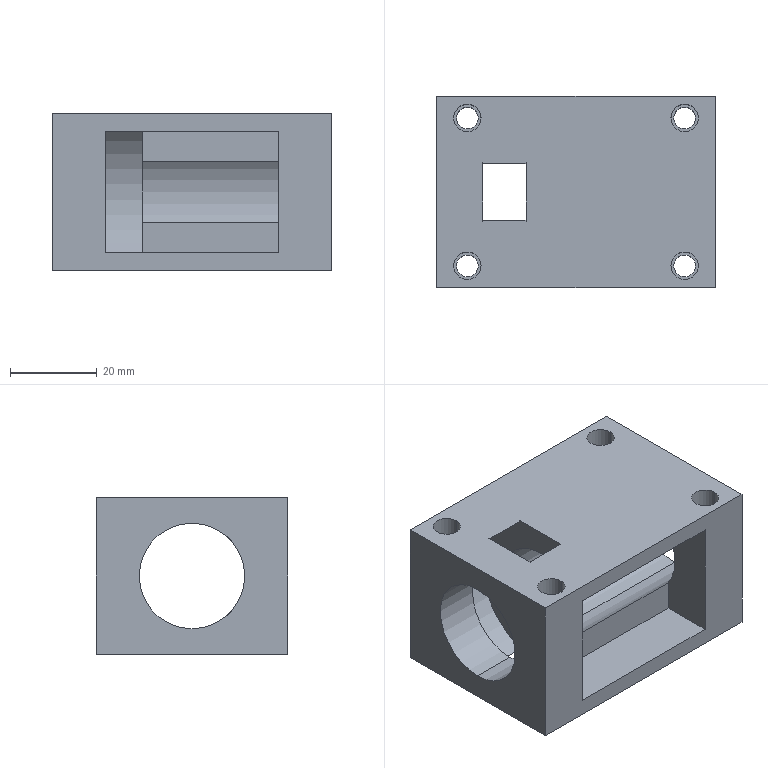Part | SolidWorks | features BaseBody 1 | 1 solid | 40 faces | box 64 x 44 x 36 mm | volume 50225 mm3 | cylinder 22 | plane 18 | commonest cylinder face diameters 5 x8 6.3 x8 24.3 x4 38.3 x2
STEP:
#1=CARTESIAN_POINT('',(-11.5,0.,30.15));
#2=VERTEX_POINT('',#1);
#3=CARTESIAN_POINT('',(-11.5,-10.,24.901));
#4=VERTEX_POINT('',#3);
#5=CARTESIAN_POINT('',(-11.5,0.,18.));
#6=DIRECTION('',(1.,0.,0.));
#7=DIRECTION('',(0.,0.,-1.));
#8=AXIS2_PLACEMENT_3D('',#5,#6,#7);
#9=CIRCLE('',#8,12.15);
#10=EDGE_CURVE('',#2,#4,#9,.T.);
#11=ORIENTED_EDGE('',*,*,#10,.F.);
#12=CARTESIAN_POINT('',(32.,0.,30.15));
#13=VERTEX_POINT('',#12);
#14=CARTESIAN_POINT('',(-33.,0.,30.15));
#15=DIRECTION('',(1.,0.,0.));
#16=VECTOR('',#15,1000.);
#17=LINE('',#14,#16);
#18=EDGE_CURVE('',#2,#13,#17,.T.);
#19=ORIENTED_EDGE('',*,*,#18,.T.);
#20=CARTESIAN_POINT('',(32.,0.,5.85));
#21=VERTEX_POINT('',#20);
#22=CARTESIAN_POINT('',(32.,0.,18.));
#23=DIRECTION('',(-1.,0.,0.));
#24=DIRECTION('',(0.,0.,-1.));
#25=AXIS2_PLACEMENT_3D('',#22,#23,#24);
#26=CIRCLE('',#25,12.15);
#27=EDGE_CURVE('',#21,#13,#26,.T.);
#28=ORIENTED_EDGE('',*,*,#27,.F.);
#29=CARTESIAN_POINT('',(-11.5,0.,5.85));
#30=VERTEX_POINT('',#29);
#31=CARTESIAN_POINT('',(-33.,0.,5.85));
#32=DIRECTION('',(1.,0.,0.));
#33=VECTOR('',#32,1000.);
#34=LINE('',#31,#33);
#35=EDGE_CURVE('',#30,#21,#34,.T.);
#36=ORIENTED_EDGE('',*,*,#35,.F.);
#37=CARTESIAN_POINT('',(-11.5,-10.,11.099));
#38=VERTEX_POINT('',#37);
#39=CARTESIAN_POINT('',(-11.5,0.,18.));
#40=DIRECTION('',(1.,0.,0.));
#41=DIRECTION('',(0.,0.,-1.));
#42=AXIS2_PLACEMENT_3D('',#39,#40,#41);
#43=CIRCLE('',#42,12.15);
#44=EDGE_CURVE('',#38,#30,#43,.T.);
#45=ORIENTED_EDGE('',*,*,#44,.F.);
#46=CARTESIAN_POINT('',(20.,-10.,11.099));
#47=VERTEX_POINT('',#46);
#48=CARTESIAN_POINT('',(-33.,-10.,11.099));
#49=DIRECTION('',(-1.,0.,0.));
#50=VECTOR('',#49,1000.);
#51=LINE('',#48,#50);
#52=EDGE_CURVE('',#47,#38,#51,.T.);
#53=ORIENTED_EDGE('',*,*,#52,.F.);
#54=CARTESIAN_POINT('',(20.,-10.,24.901));
#55=VERTEX_POINT('',#54);
#56=CARTESIAN_POINT('',(20.,0.,18.));
#57=DIRECTION('',(1.,0.,0.));
#58=DIRECTION('',(0.,0.,-1.));
#59=AXIS2_PLACEMENT_3D('',#56,#57,#58);
#60=CIRCLE('',#59,12.15);
#61=EDGE_CURVE('',#55,#47,#60,.T.);
#62=ORIENTED_EDGE('',*,*,#61,.F.);
#63=CARTESIAN_POINT('',(-33.,-10.,24.901));
#64=DIRECTION('',(1.,0.,0.));
#65=VECTOR('',#64,1000.);
#66=LINE('',#63,#65);
#67=EDGE_CURVE('',#4,#55,#66,.T.);
#68=ORIENTED_EDGE('',*,*,#67,.F.);
#69=EDGE_LOOP('',(#11,#19,#28,#36,#45,#53,#62,#68));
#70=FACE_OUTER_BOUND('',#69,.T.);
#71=CARTESIAN_POINT('',(-33.,0.,18.));
#72=DIRECTION('',(1.,0.,0.));
#73=DIRECTION('',(0.,0.,-1.));
#74=AXIS2_PLACEMENT_3D('',#71,#72,#73);
#75=CYLINDRICAL_SURFACE('',#74,12.15);
#76=ADVANCED_FACE('',(#70),#75,.F.);
#77=CARTESIAN_POINT('',(21.85,17.,16.8));
#78=VERTEX_POINT('',#77);
#79=CARTESIAN_POINT('',(28.15,17.,16.8));
#80=VERTEX_POINT('',#79);
#81=CARTESIAN_POINT('',(25.,17.,16.8));
#82=DIRECTION('',(0.,0.,1.));
#83=DIRECTION('',(1.,0.,0.));
#84=AXIS2_PLACEMENT_3D('',#81,#82,#83);
#85=CIRCLE('',#84,3.15);
#86=EDGE_CURVE('',#78,#80,#85,.T.);
#87=ORIENTED_EDGE('',*,*,#86,.F.);
#88=CARTESIAN_POINT('',(21.85,17.,36.));
#89=VERTEX_POINT('',#88);
#90=CARTESIAN_POINT('',(21.85,17.,16.8));
#91=DIRECTION('',(0.,0.,1.));
#92=VECTOR('',#91,1000.);
#93=LINE('',#90,#92);
#94=EDGE_CURVE('',#78,#89,#93,.T.);
#95=ORIENTED_EDGE('',*,*,#94,.T.);
#96=CARTESIAN_POINT('',(28.15,17.,36.));
#97=VERTEX_POINT('',#96);
#98=CARTESIAN_POINT('',(25.,17.,36.));
#99=DIRECTION('',(0.,0.,-1.));
#100=DIRECTION('',(1.,0.,0.));
#101=AXIS2_PLACEMENT_3D('',#98,#99,#100);
#102=CIRCLE('',#101,3.15);
#103=EDGE_CURVE('',#97,#89,#102,.T.);
#104=ORIENTED_EDGE('',*,*,#103,.F.);
#105=CARTESIAN_POINT('',(28.15,17.,16.8));
#106=DIRECTION('',(0.,0.,1.));
#107=VECTOR('',#106,1000.);
#108=LINE('',#105,#107);
#109=EDGE_CURVE('',#80,#97,#108,.T.);
#110=ORIENTED_EDGE('',*,*,#109,.F.);
#111=EDGE_LOOP('',(#87,#95,#104,#110));
#112=FACE_OUTER_BOUND('',#111,.T.);
#113=CARTESIAN_POINT('',(25.,17.,16.8));
#114=DIRECTION('',(0.,0.,1.));
#115=DIRECTION('',(1.,0.,0.));
#116=AXIS2_PLACEMENT_3D('',#113,#114,#115);
#117=CYLINDRICAL_SURFACE('',#116,3.15);
#118=ADVANCED_FACE('',(#112),#117,.F.);
#119=CARTESIAN_POINT('',(-28.15,17.,16.8));
#120=VERTEX_POINT('',#119);
#121=CARTESIAN_POINT('',(-21.85,17.,16.8));
#122=VERTEX_POINT('',#121);
#123=CARTESIAN_POINT('',(-25.,17.,16.8));
#124=DIRECTION('',(0.,0.,1.));
#125=DIRECTION('',(1.,0.,0.));
#126=AXIS2_PLACEMENT_3D('',#123,#124,#125);
#127=CIRCLE('',#126,3.15);
#128=EDGE_CURVE('',#120,#122,#127,.T.);
#129=ORIENTED_EDGE('',*,*,#128,.F.);
#130=CARTESIAN_POINT('',(-28.15,17.,36.));
#131=VERTEX_POINT('',#130);
#132=CARTESIAN_POINT('',(-28.15,17.,16.8));
#133=DIRECTION('',(0.,0.,1.));
#134=VECTOR('',#133,1000.);
#135=LINE('',#132,#134);
#136=EDGE_CURVE('',#120,#131,#135,.T.);
#137=ORIENTED_EDGE('',*,*,#136,.T.);
#138=CARTESIAN_POINT('',(-21.85,17.,36.));
#139=VERTEX_POINT('',#138);
#140=CARTESIAN_POINT('',(-25.,17.,36.));
#141=DIRECTION('',(0.,0.,-1.));
#142=DIRECTION('',(1.,0.,0.));
#143=AXIS2_PLACEMENT_3D('',#140,#141,#142);
#144=CIRCLE('',#143,3.15);
#145=EDGE_CURVE('',#139,#131,#144,.T.);
#146=ORIENTED_EDGE('',*,*,#145,.F.);
#147=CARTESIAN_POINT('',(-21.85,17.,16.8));
#148=DIRECTION('',(0.,0.,1.));
#149=VECTOR('',#148,1000.);
#150=LINE('',#147,#149);
#151=EDGE_CURVE('',#122,#139,#150,.T.);
#152=ORIENTED_EDGE('',*,*,#151,.F.);
#153=EDGE_LOOP('',(#129,#137,#146,#152));
#154=FACE_OUTER_BOUND('',#153,.T.);
#155=CARTESIAN_POINT('',(-25.,17.,16.8));
#156=DIRECTION('',(0.,0.,1.));
#157=DIRECTION('',(1.,0.,0.));
#158=AXIS2_PLACEMENT_3D('',#155,#156,#157);
#159=CYLINDRICAL_SURFACE('',#158,3.15);
#160=ADVANCED_FACE('',(#154),#159,.F.);
#161=CARTESIAN_POINT('',(21.85,-17.,16.8));
#162=VERTEX_POINT('',#161);
#163=CARTESIAN_POINT('',(28.15,-17.,16.8));
#164=VERTEX_POINT('',#163);
#165=CARTESIAN_POINT('',(25.,-17.,16.8));
#166=DIRECTION('',(0.,0.,1.));
#167=DIRECTION('',(1.,0.,0.));
#168=AXIS2_PLACEMENT_3D('',#165,#166,#167);
#169=CIRCLE('',#168,3.15);
#170=EDGE_CURVE('',#162,#164,#169,.T.);
#171=ORIENTED_EDGE('',*,*,#170,.F.);
#172=CARTESIAN_POINT('',(21.85,-17.,36.));
#173=VERTEX_POINT('',#172);
#174=CARTESIAN_POINT('',(21.85,-17.,16.8));
#175=DIRECTION('',(0.,0.,1.));
#176=VECTOR('',#175,1000.);
#177=LINE('',#174,#176);
#178=EDGE_CURVE('',#162,#173,#177,.T.);
#179=ORIENTED_EDGE('',*,*,#178,.T.);
#180=CARTESIAN_POINT('',(28.15,-17.,36.));
#181=VERTEX_POINT('',#180);
#182=CARTESIAN_POINT('',(25.,-17.,36.));
#183=DIRECTION('',(0.,0.,-1.));
#184=DIRECTION('',(1.,0.,0.));
#185=AXIS2_PLACEMENT_3D('',#182,#183,#184);
#186=CIRCLE('',#185,3.15);
#187=EDGE_CURVE('',#181,#173,#186,.T.);
#188=ORIENTED_EDGE('',*,*,#187,.F.);
#189=CARTESIAN_POINT('',(28.15,-17.,16.8));
#190=DIRECTION('',(0.,0.,1.));
#191=VECTOR('',#190,1000.);
#192=LINE('',#189,#191);
#193=EDGE_CURVE('',#164,#181,#192,.T.);
#194=ORIENTED_EDGE('',*,*,#193,.F.);
#195=EDGE_LOOP('',(#171,#179,#188,#194));
#196=FACE_OUTER_BOUND('',#195,.T.);
#197=CARTESIAN_POINT('',(25.,-17.,16.8));
#198=DIRECTION('',(0.,0.,1.));
#199=DIRECTION('',(1.,0.,0.));
#200=AXIS2_PLACEMENT_3D('',#197,#198,#199);
#201=CYLINDRICAL_SURFACE('',#200,3.15);
#202=ADVANCED_FACE('',(#196),#201,.F.);
#203=CARTESIAN_POINT('',(-28.15,-17.,16.8));
#204=VERTEX_POINT('',#203);
#205=CARTESIAN_POINT('',(-21.85,-17.,16.8));
#206=VERTEX_POINT('',#205);
#207=CARTESIAN_POINT('',(-25.,-17.,16.8));
#208=DIRECTION('',(0.,0.,1.));
#209=DIRECTION('',(1.,0.,0.));
#210=AXIS2_PLACEMENT_3D('',#207,#208,#209);
#211=CIRCLE('',#210,3.15);
#212=EDGE_CURVE('',#204,#206,#211,.T.);
#213=ORIENTED_EDGE('',*,*,#212,.F.);
#214=CARTESIAN_POINT('',(-28.15,-17.,36.));
#215=VERTEX_POINT('',#214);
#216=CARTESIAN_POINT('',(-28.15,-17.,16.8));
#217=DIRECTION('',(0.,0.,1.));
#218=VECTOR('',#217,1000.);
#219=LINE('',#216,#218);
#220=EDGE_CURVE('',#204,#215,#219,.T.);
#221=ORIENTED_EDGE('',*,*,#220,.T.);
#222=CARTESIAN_POINT('',(-21.85,-17.,36.));
#223=VERTEX_POINT('',#222);
#224=CARTESIAN_POINT('',(-25.,-17.,36.));
#225=DIRECTION('',(0.,0.,-1.));
#226=DIRECTION('',(1.,0.,0.));
#227=AXIS2_PLACEMENT_3D('',#224,#225,#226);
#228=CIRCLE('',#227,3.15);
#229=EDGE_CURVE('',#223,#215,#228,.T.);
#230=ORIENTED_EDGE('',*,*,#229,.F.);
#231=CARTESIAN_POINT('',(-21.85,-17.,16.8));
#232=DIRECTION('',(0.,0.,1.));
#233=VECTOR('',#232,1000.);
#234=LINE('',#231,#233);
#235=EDGE_CURVE('',#206,#223,#234,.T.);
#236=ORIENTED_EDGE('',*,*,#235,.F.);
#237=EDGE_LOOP('',(#213,#221,#230,#236));
#238=FACE_OUTER_BOUND('',#237,.T.);
#239=CARTESIAN_POINT('',(-25.,-17.,16.8));
#240=DIRECTION('',(0.,0.,1.));
#241=DIRECTION('',(1.,0.,0.));
#242=AXIS2_PLACEMENT_3D('',#239,#240,#241);
#243=CYLINDRICAL_SURFACE('',#242,3.15);
#244=ADVANCED_FACE('',(#238),#243,.F.);
#245=CARTESIAN_POINT('',(27.5,17.,0.));
#246=VERTEX_POINT('',#245);
#247=CARTESIAN_POINT('',(22.5,17.,0.));
#248=VERTEX_POINT('',#247);
#249=CARTESIAN_POINT('',(25.,17.,0.));
#250=DIRECTION('',(0.,0.,-1.));
#251=DIRECTION('',(1.,0.,0.));
#252=AXIS2_PLACEMENT_3D('',#249,#250,#251);
#253=CIRCLE('',#252,2.5);
#254=EDGE_CURVE('',#246,#248,#253,.T.);
#255=ORIENTED_EDGE('',*,*,#254,.T.);
#256=CARTESIAN_POINT('',(22.5,17.,16.8));
#257=VERTEX_POINT('',#256);
#258=CARTESIAN_POINT('',(22.5,17.,-2.));
#259=DIRECTION('',(0.,0.,1.));
#260=VECTOR('',#259,1000.);
#261=LINE('',#258,#260);
#262=EDGE_CURVE('',#248,#257,#261,.T.);
#263=ORIENTED_EDGE('',*,*,#262,.T.);
#264=CARTESIAN_POINT('',(27.5,17.,16.8));
#265=VERTEX_POINT('',#264);
#266=CARTESIAN_POINT('',(25.,17.,16.8));
#267=DIRECTION('',(0.,0.,-1.));
#268=DIRECTION('',(1.,0.,0.));
#269=AXIS2_PLACEMENT_3D('',#266,#267,#268);
#270=CIRCLE('',#269,2.5);
#271=EDGE_CURVE('',#265,#257,#270,.T.);
#272=ORIENTED_EDGE('',*,*,#271,.F.);
#273=CARTESIAN_POINT('',(27.5,17.,-2.));
#274=DIRECTION('',(0.,0.,1.));
#275=VECTOR('',#274,1000.);
#276=LINE('',#273,#275);
#277=EDGE_CURVE('',#246,#265,#276,.T.);
#278=ORIENTED_EDGE('',*,*,#277,.F.);
#279=EDGE_LOOP('',(#255,#263,#272,#278));
#280=FACE_OUTER_BOUND('',#279,.T.);
#281=CARTESIAN_POINT('',(25.,17.,-2.));
#282=DIRECTION('',(0.,0.,1.));
#283=DIRECTION('',(1.,0.,0.));
#284=AXIS2_PLACEMENT_3D('',#281,#282,#283);
#285=CYLINDRICAL_SURFACE('',#284,2.5);
#286=ADVANCED_FACE('',(#280),#285,.F.);
#287=CARTESIAN_POINT('',(-22.5,17.,0.));
#288=VERTEX_POINT('',#287);
#289=CARTESIAN_POINT('',(-27.5,17.,0.));
#290=VERTEX_POINT('',#289);
#291=CARTESIAN_POINT('',(-25.,17.,0.));
#292=DIRECTION('',(0.,0.,-1.));
#293=DIRECTION('',(1.,0.,0.));
#294=AXIS2_PLACEMENT_3D('',#291,#292,#293);
#295=CIRCLE('',#294,2.5);
#296=EDGE_CURVE('',#288,#290,#295,.T.);
#297=ORIENTED_EDGE('',*,*,#296,.T.);
#298=CARTESIAN_POINT('',(-27.5,17.,16.8));
#299=VERTEX_POINT('',#298);
#300=CARTESIAN_POINT('',(-27.5,17.,-2.));
#301=DIRECTION('',(0.,0.,1.));
#302=VECTOR('',#301,1000.);
#303=LINE('',#300,#302);
#304=EDGE_CURVE('',#290,#299,#303,.T.);
#305=ORIENTED_EDGE('',*,*,#304,.T.);
#306=CARTESIAN_POINT('',(-22.5,17.,16.8));
#307=VERTEX_POINT('',#306);
#308=CARTESIAN_POINT('',(-25.,17.,16.8));
#309=DIRECTION('',(0.,0.,-1.));
#310=DIRECTION('',(1.,0.,0.));
#311=AXIS2_PLACEMENT_3D('',#308,#309,#310);
#312=CIRCLE('',#311,2.5);
#313=EDGE_CURVE('',#307,#299,#312,.T.);
#314=ORIENTED_EDGE('',*,*,#313,.F.);
#315=CARTESIAN_POINT('',(-22.5,17.,-2.));
#316=DIRECTION('',(0.,0.,1.));
#317=VECTOR('',#316,1000.);
#318=LINE('',#315,#317);
#319=EDGE_CURVE('',#288,#307,#318,.T.);
#320=ORIENTED_EDGE('',*,*,#319,.F.);
#321=EDGE_LOOP('',(#297,#305,#314,#320));
#322=FACE_OUTER_BOUND('',#321,.T.);
#323=CARTESIAN_POINT('',(-25.,17.,-2.));
#324=DIRECTION('',(0.,0.,1.));
#325=DIRECTION('',(1.,0.,0.));
#326=AXIS2_PLACEMENT_3D('',#323,#324,#325);
#327=CYLINDRICAL_SURFACE('',#326,2.5);
#328=ADVANCED_FACE('',(#322),#327,.F.);
#329=CARTESIAN_POINT('',(27.5,-17.,0.));
#330=VERTEX_POINT('',#329);
#331=CARTESIAN_POINT('',(22.5,-17.,0.));
#332=VERTEX_POINT('',#331);
#333=CARTESIAN_POINT('',(25.,-17.,0.));
#334=DIRECTION('',(0.,0.,-1.));
#335=DIRECTION('',(1.,0.,0.));
#336=AXIS2_PLACEMENT_3D('',#333,#334,#335);
#337=CIRCLE('',#336,2.5);
#338=EDGE_CURVE('',#330,#332,#337,.T.);
#339=ORIENTED_EDGE('',*,*,#338,.T.);
#340=CARTESIAN_POINT('',(22.5,-17.,16.8));
#341=VERTEX_POINT('',#340);
#342=CARTESIAN_POINT('',(22.5,-17.,-2.));
#343=DIRECTION('',(0.,0.,1.));
#344=VECTOR('',#343,1000.);
#345=LINE('',#342,#344);
#346=EDGE_CURVE('',#332,#341,#345,.T.);
#347=ORIENTED_EDGE('',*,*,#346,.T.);
#348=CARTESIAN_POINT('',(27.5,-17.,16.8));
#349=VERTEX_POINT('',#348);
#350=CARTESIAN_POINT('',(25.,-17.,16.8));
#351=DIRECTION('',(0.,0.,-1.));
#352=DIRECTION('',(1.,0.,0.));
#353=AXIS2_PLACEMENT_3D('',#350,#351,#352);
#354=CIRCLE('',#353,2.5);
#355=EDGE_CURVE('',#349,#341,#354,.T.);
#356=ORIENTED_EDGE('',*,*,#355,.F.);
#357=CARTESIAN_POINT('',(27.5,-17.,-2.));
#358=DIRECTION('',(0.,0.,1.));
#359=VECTOR('',#358,1000.);
#360=LINE('',#357,#359);
#361=EDGE_CURVE('',#330,#349,#360,.T.);
#362=ORIENTED_EDGE('',*,*,#361,.F.);
#363=EDGE_LOOP('',(#339,#347,#356,#362));
#364=FACE_OUTER_BOUND('',#363,.T.);
#365=CARTESIAN_POINT('',(25.,-17.,-2.));
#366=DIRECTION('',(0.,0.,1.));
#367=DIRECTION('',(1.,0.,0.));
#368=AXIS2_PLACEMENT_3D('',#365,#366,#367);
#369=CYLINDRICAL_SURFACE('',#368,2.5);
#370=ADVANCED_FACE('',(#364),#369,.F.);
#371=CARTESIAN_POINT('',(-22.5,-17.,0.));
#372=VERTEX_POINT('',#371);
#373=CARTESIAN_POINT('',(-27.5,-17.,0.));
#374=VERTEX_POINT('',#373);
#375=CARTESIAN_POINT('',(-25.,-17.,0.));
#376=DIRECTION('',(0.,0.,-1.));
#377=DIRECTION('',(1.,0.,0.));
#378=AXIS2_PLACEMENT_3D('',#375,#376,#377);
#379=CIRCLE('',#378,2.5);
#380=EDGE_CURVE('',#372,#374,#379,.T.);
#381=ORIENTED_EDGE('',*,*,#380,.T.);
#382=CARTESIAN_POINT('',(-27.5,-17.,16.8));
#383=VERTEX_POINT('',#382);
#384=CARTESIAN_POINT('',(-27.5,-17.,-2.));
#385=DIRECTION('',(0.,0.,1.));
#386=VECTOR('',#385,1000.);
#387=LINE('',#384,#386);
#388=EDGE_CURVE('',#374,#383,#387,.T.);
#389=ORIENTED_EDGE('',*,*,#388,.T.);
#390=CARTESIAN_POINT('',(-22.5,-17.,16.8));
#391=VERTEX_POINT('',#390);
#392=CARTESIAN_POINT('',(-25.,-17.,16.8));
#393=DIRECTION('',(0.,0.,-1.));
#394=DIRECTION('',(1.,0.,0.));
#395=AXIS2_PLACEMENT_3D('',#392,#393,#394);
#396=CIRCLE('',#395,2.5);
#397=EDGE_CURVE('',#391,#383,#396,.T.);
#398=ORIENTED_EDGE('',*,*,#397,.F.);
#399=CARTESIAN_POINT('',(-22.5,-17.,-2.));
#400=DIRECTION('',(0.,0.,1.));
#401=VECTOR('',#400,1000.);
#402=LINE('',#399,#401);
#403=EDGE_CURVE('',#372,#391,#402,.T.);
#404=ORIENTED_EDGE('',*,*,#403,.F.);
#405=EDGE_LOOP('',(#381,#389,#398,#404));
#406=FACE_OUTER_BOUND('',#405,.T.);
#407=CARTESIAN_POINT('',(-25.,-17.,-2.));
#408=DIRECTION('',(0.,0.,1.));
#409=DIRECTION('',(1.,0.,0.));
#410=AXIS2_PLACEMENT_3D('',#407,#408,#409);
#411=CYLINDRICAL_SURFACE('',#410,2.5);
#412=ADVANCED_FACE('',(#406),#411,.F.);
#413=CARTESIAN_POINT('',(-32.,0.,5.85));
#414=VERTEX_POINT('',#413);
#415=CARTESIAN_POINT('',(-32.,0.,30.15));
#416=VERTEX_POINT('',#415);
#417=CARTESIAN_POINT('',(-32.,0.,18.));
#418=DIRECTION('',(-1.,0.,0.));
#419=DIRECTION('',(0.,0.,-1.));
#420=AXIS2_PLACEMENT_3D('',#417,#418,#419);
#421=CIRCLE('',#420,12.15);
#422=EDGE_CURVE('',#414,#416,#421,.T.);
#423=ORIENTED_EDGE('',*,*,#422,.T.);
#424=CARTESIAN_POINT('',(-21.5,0.,30.15));
#425=VERTEX_POINT('',#424);
#426=CARTESIAN_POINT('',(-33.,0.,30.15));
#427=DIRECTION('',(1.,0.,0.));
#428=VECTOR('',#427,1000.);
#429=LINE('',#426,#428);
#430=EDGE_CURVE('',#416,#425,#429,.T.);
#431=ORIENTED_EDGE('',*,*,#430,.T.);
#432=CARTESIAN_POINT('',(-21.5,0.,5.85));
#433=VERTEX_POINT('',#432);
#434=CARTESIAN_POINT('',(-21.5,0.,18.));
#435=DIRECTION('',(-1.,0.,0.));
#436=DIRECTION('',(0.,0.,-1.));
#437=AXIS2_PLACEMENT_3D('',#434,#435,#436);
#438=CIRCLE('',#437,12.15);
#439=EDGE_CURVE('',#433,#425,#438,.T.);
#440=ORIENTED_EDGE('',*,*,#439,.F.);
#441=CARTESIAN_POINT('',(-33.,0.,5.85));
#442=DIRECTION('',(1.,0.,0.));
#443=VECTOR('',#442,1000.);
#444=LINE('',#441,#443);
#445=EDGE_CURVE('',#414,#433,#444,.T.);
#446=ORIENTED_EDGE('',*,*,#445,.F.);
#447=EDGE_LOOP('',(#423,#431,#440,#446));
#448=FACE_OUTER_BOUND('',#447,.T.);
#449=CARTESIAN_POINT('',(-33.,0.,18.));
#450=DIRECTION('',(1.,0.,0.));
#451=DIRECTION('',(0.,0.,-1.));
#452=AXIS2_PLACEMENT_3D('',#449,#450,#451);
#453=CYLINDRICAL_SURFACE('',#452,12.15);
#454=ADVANCED_FACE('',(#448),#453,.F.);
#455=ORIENTED_EDGE('',*,*,#18,.F.);
#456=CARTESIAN_POINT('',(-11.5,0.,18.));
#457=DIRECTION('',(1.,0.,0.));
#458=DIRECTION('',(0.,0.,-1.));
#459=AXIS2_PLACEMENT_3D('',#456,#457,#458);
#460=CIRCLE('',#459,12.15);
#461=EDGE_CURVE('',#30,#2,#460,.T.);
#462=ORIENTED_EDGE('',*,*,#461,.F.);
#463=ORIENTED_EDGE('',*,*,#35,.T.);
#464=CARTESIAN_POINT('',(32.,0.,18.));
#465=DIRECTION('',(-1.,0.,0.));
#466=DIRECTION('',(0.,0.,-1.));
#467=AXIS2_PLACEMENT_3D('',#464,#465,#466);
#468=CIRCLE('',#467,12.15);
#469=EDGE_CURVE('',#13,#21,#468,.T.);
#470=ORIENTED_EDGE('',*,*,#469,.F.);
#471=EDGE_LOOP('',(#455,#462,#463,#470));
#472=FACE_OUTER_BOUND('',#471,.T.);
#473=CARTESIAN_POINT('',(-33.,0.,18.));
#474=DIRECTION('',(1.,0.,0.));
#475=DIRECTION('',(0.,0.,-1.));
#476=AXIS2_PLACEMENT_3D('',#473,#474,#475);
#477=CYLINDRICAL_SURFACE('',#476,12.15);
#478=ADVANCED_FACE('',(#472),#477,.F.);
#479=ORIENTED_EDGE('',*,*,#61,.T.);
#480=CARTESIAN_POINT('',(20.,-10.,4.));
#481=VERTEX_POINT('',#480);
#482=CARTESIAN_POINT('',(20.,-10.,4.));
#483=DIRECTION('',(0.,0.,1.));
#484=VECTOR('',#483,1000.);
#485=LINE('',#482,#484);
#486=EDGE_CURVE('',#481,#47,#485,.T.);
#487=ORIENTED_EDGE('',*,*,#486,.F.);
#488=CARTESIAN_POINT('',(20.,-22.,4.));
#489=VERTEX_POINT('',#488);
#490=CARTESIAN_POINT('',(20.,-32.,4.));
#491=DIRECTION('',(0.,1.,0.));
#492=VECTOR('',#491,1000.);
#493=LINE('',#490,#492);
#494=EDGE_CURVE('',#489,#481,#493,.T.);
#495=ORIENTED_EDGE('',*,*,#494,.F.);
#496=CARTESIAN_POINT('',(20.,-22.,32.));
#497=VERTEX_POINT('',#496);
#498=CARTESIAN_POINT('',(20.,-22.,4.));
#499=DIRECTION('',(0.,0.,-1.));
#500=VECTOR('',#499,1000.);
#501=LINE('',#498,#500);
#502=EDGE_CURVE('',#497,#489,#501,.T.);
#503=ORIENTED_EDGE('',*,*,#502,.F.);
#504=CARTESIAN_POINT('',(20.,-10.,32.));
#505=VERTEX_POINT('',#504);
#506=CARTESIAN_POINT('',(20.,-32.,32.));
#507=DIRECTION('',(0.,-1.,0.));
#508=VECTOR('',#507,1000.);
#509=LINE('',#506,#508);
#510=EDGE_CURVE('',#505,#497,#509,.T.);
#511=ORIENTED_EDGE('',*,*,#510,.F.);
#512=CARTESIAN_POINT('',(20.,-10.,4.));
#513=DIRECTION('',(0.,0.,1.));
#514=VECTOR('',#513,1000.);
#515=LINE('',#512,#514);
#516=EDGE_CURVE('',#55,#505,#515,.T.);
#517=ORIENTED_EDGE('',*,*,#516,.F.);
#518=EDGE_LOOP('',(#479,#487,#495,#503,#511,#517));
#519=FACE_OUTER_BOUND('',#518,.T.);
#520=CARTESIAN_POINT('',(20.,-32.,4.));
#521=DIRECTION('',(1.,0.,0.));
#522=DIRECTION('',(0.,0.,-1.));
#523=AXIS2_PLACEMENT_3D('',#520,#521,#522);
#524=PLANE('',#523);
#525=ADVANCED_FACE('',(#519),#524,.F.);
#526=ORIENTED_EDGE('',*,*,#516,.T.);
#527=CARTESIAN_POINT('',(-11.5,-10.,32.));
#528=VERTEX_POINT('',#527);
#529=CARTESIAN_POINT('',(-20.,-10.,32.));
#530=DIRECTION('',(1.,0.,0.));
#531=VECTOR('',#530,1000.);
#532=LINE('',#529,#531);
#533=EDGE_CURVE('',#528,#505,#532,.T.);
#534=ORIENTED_EDGE('',*,*,#533,.F.);
#535=CARTESIAN_POINT('',(-11.5,-10.,4.));
#536=DIRECTION('',(0.,0.,1.));
#537=VECTOR('',#536,1000.);
#538=LINE('',#535,#537);
#539=EDGE_CURVE('',#4,#528,#538,.T.);
#540=ORIENTED_EDGE('',*,*,#539,.F.);
#541=ORIENTED_EDGE('',*,*,#67,.T.);
#542=EDGE_LOOP('',(#526,#534,#540,#541));
#543=FACE_OUTER_BOUND('',#542,.T.);
#544=CARTESIAN_POINT('',(-20.,-10.,4.));
#545=DIRECTION('',(0.,1.,0.));
#546=DIRECTION('',(0.,0.,1.));
#547=AXIS2_PLACEMENT_3D('',#544,#545,#546);
#548=PLANE('',#547);
#549=ADVANCED_FACE('',(#543),#548,.F.);
#550=CARTESIAN_POINT('',(-11.5,-10.,4.));
#551=VERTEX_POINT('',#550);
#552=CARTESIAN_POINT('',(-11.5,-10.,18.));
#553=DIRECTION('',(0.,0.,-1.));
#554=VECTOR('',#553,1000.);
#555=LINE('',#552,#554);
#556=EDGE_CURVE('',#38,#551,#555,.T.);
#557=ORIENTED_EDGE('',*,*,#556,.F.);
#558=ORIENTED_EDGE('',*,*,#44,.T.);
#559=ORIENTED_EDGE('',*,*,#461,.T.);
#560=ORIENTED_EDGE('',*,*,#10,.T.);
#561=ORIENTED_EDGE('',*,*,#539,.T.);
#562=CARTESIAN_POINT('',(-11.5,-13.066,32.));
#563=VERTEX_POINT('',#562);
#564=CARTESIAN_POINT('',(-11.5,0.,32.));
#565=DIRECTION('',(0.,1.,0.));
#566=VECTOR('',#565,1000.);
#567=LINE('',#564,#566);
#568=EDGE_CURVE('',#563,#528,#567,.T.);
#569=ORIENTED_EDGE('',*,*,#568,.F.);
#570=CARTESIAN_POINT('',(-11.5,-6.536,36.));
#571=VERTEX_POINT('',#570);
#572=CARTESIAN_POINT('',(-11.5,0.,18.));
#573=DIRECTION('',(1.,0.,0.));
#574=DIRECTION('',(0.,0.,-1.));
#575=AXIS2_PLACEMENT_3D('',#572,#573,#574);
#576=CIRCLE('',#575,19.15);
#577=EDGE_CURVE('',#571,#563,#576,.T.);
#578=ORIENTED_EDGE('',*,*,#577,.F.);
#579=CARTESIAN_POINT('',(-11.5,6.536,36.));
#580=VERTEX_POINT('',#579);
#581=CARTESIAN_POINT('',(-11.5,0.,36.));
#582=DIRECTION('',(0.,-1.,0.));
#583=VECTOR('',#582,1000.);
#584=LINE('',#581,#583);
#585=EDGE_CURVE('',#580,#571,#584,.T.);
#586=ORIENTED_EDGE('',*,*,#585,.F.);
#587=CARTESIAN_POINT('',(-11.5,6.536,0.));
#588=VERTEX_POINT('',#587);
#589=CARTESIAN_POINT('',(-11.5,0.,18.));
#590=DIRECTION('',(1.,0.,0.));
#591=DIRECTION('',(0.,0.,-1.));
#592=AXIS2_PLACEMENT_3D('',#589,#590,#591);
#593=CIRCLE('',#592,19.15);
#594=EDGE_CURVE('',#588,#580,#593,.T.);
#595=ORIENTED_EDGE('',*,*,#594,.F.);
#596=CARTESIAN_POINT('',(-11.5,-6.536,0.));
#597=VERTEX_POINT('',#596);
#598=CARTESIAN_POINT('',(-11.5,0.,0.));
#599=DIRECTION('',(0.,1.,0.));
#600=VECTOR('',#599,1000.);
#601=LINE('',#598,#600);
#602=EDGE_CURVE('',#597,#588,#601,.T.);
#603=ORIENTED_EDGE('',*,*,#602,.F.);
#604=CARTESIAN_POINT('',(-11.5,-13.066,4.));
#605=VERTEX_POINT('',#604);
#606=CARTESIAN_POINT('',(-11.5,0.,18.));
#607=DIRECTION('',(1.,0.,0.));
#608=DIRECTION('',(0.,0.,-1.));
#609=AXIS2_PLACEMENT_3D('',#606,#607,#608);
#610=CIRCLE('',#609,19.15);
#611=EDGE_CURVE('',#605,#597,#610,.T.);
#612=ORIENTED_EDGE('',*,*,#611,.F.);
#613=CARTESIAN_POINT('',(-11.5,0.,4.));
#614=DIRECTION('',(0.,-1.,0.));
#615=VECTOR('',#614,1000.);
#616=LINE('',#613,#615);
#617=EDGE_CURVE('',#551,#605,#616,.T.);
#618=ORIENTED_EDGE('',*,*,#617,.F.);
#619=EDGE_LOOP('',(#557,#558,#559,#560,#561,#569,#578,#586,#595,#603,#612,#618));
#620=FACE_OUTER_BOUND('',#619,.T.);
#621=CARTESIAN_POINT('',(-11.5,0.,18.));
#622=DIRECTION('',(1.,0.,0.));
#623=DIRECTION('',(0.,0.,-1.));
#624=AXIS2_PLACEMENT_3D('',#621,#622,#623);
#625=PLANE('',#624);
#626=ADVANCED_FACE('',(#620),#625,.F.);
#627=ORIENTED_EDGE('',*,*,#27,.T.);
#628=ORIENTED_EDGE('',*,*,#469,.T.);
#629=EDGE_LOOP('',(#627,#628));
#630=FACE_BOUND('',#629,.T.);
#631=CARTESIAN_POINT('',(32.,22.,0.));
#632=VERTEX_POINT('',#631);
#633=CARTESIAN_POINT('',(32.,22.,36.));
#634=VERTEX_POINT('',#633);
#635=CARTESIAN_POINT('',(32.,22.,0.));
#636=DIRECTION('',(0.,0.,1.));
#637=VECTOR('',#636,1000.);
#638=LINE('',#635,#637);
#639=EDGE_CURVE('',#632,#634,#638,.T.);
#640=ORIENTED_EDGE('',*,*,#639,.T.);
#641=CARTESIAN_POINT('',(32.,-22.,36.));
#642=VERTEX_POINT('',#641);
#643=CARTESIAN_POINT('',(32.,-22.,36.));
#644=DIRECTION('',(0.,-1.,0.));
#645=VECTOR('',#644,1000.);
#646=LINE('',#643,#645);
#647=EDGE_CURVE('',#634,#642,#646,.T.);
#648=ORIENTED_EDGE('',*,*,#647,.T.);
#649=CARTESIAN_POINT('',(32.,-22.,0.));
#650=VERTEX_POINT('',#649);
#651=CARTESIAN_POINT('',(32.,-22.,0.));
#652=DIRECTION('',(0.,0.,-1.));
#653=VECTOR('',#652,1000.);
#654=LINE('',#651,#653);
#655=EDGE_CURVE('',#642,#650,#654,.T.);
#656=ORIENTED_EDGE('',*,*,#655,.T.);
#657=CARTESIAN_POINT('',(32.,-22.,0.));
#658=DIRECTION('',(0.,1.,0.));
#659=VECTOR('',#658,1000.);
#660=LINE('',#657,#659);
#661=EDGE_CURVE('',#650,#632,#660,.T.);
#662=ORIENTED_EDGE('',*,*,#661,.T.);
#663=EDGE_LOOP('',(#640,#648,#656,#662));
#664=FACE_OUTER_BOUND('',#663,.T.);
#665=CARTESIAN_POINT('',(32.,-22.,0.));
#666=DIRECTION('',(1.,0.,0.));
#667=DIRECTION('',(0.,0.,-1.));
#668=AXIS2_PLACEMENT_3D('',#665,#666,#667);
#669=PLANE('',#668);
#670=ADVANCED_FACE('',(#630,#664),#669,.T.);
#671=ORIENTED_EDGE('',*,*,#52,.T.);
#672=ORIENTED_EDGE('',*,*,#556,.T.);
#673=CARTESIAN_POINT('',(-20.,-10.,4.));
#674=DIRECTION('',(-1.,0.,0.));
#675=VECTOR('',#674,1000.);
#676=LINE('',#673,#675);
#677=EDGE_CURVE('',#481,#551,#676,.T.);
#678=ORIENTED_EDGE('',*,*,#677,.F.);
#679=ORIENTED_EDGE('',*,*,#486,.T.);
#680=EDGE_LOOP('',(#671,#672,#678,#679));
#681=FACE_OUTER_BOUND('',#680,.T.);
#682=CARTESIAN_POINT('',(-20.,-10.,4.));
#683=DIRECTION('',(0.,1.,0.));
#684=DIRECTION('',(0.,0.,1.));
#685=AXIS2_PLACEMENT_3D('',#682,#683,#684);
#686=PLANE('',#685);
#687=ADVANCED_FACE('',(#681),#686,.F.);
#688=ORIENTED_EDGE('',*,*,#617,.T.);
#689=CARTESIAN_POINT('',(-20.,-13.066,4.));
#690=VERTEX_POINT('',#689);
#691=CARTESIAN_POINT('',(-20.,-13.066,4.));
#692=DIRECTION('',(-1.,0.,0.));
#693=VECTOR('',#692,1000.);
#694=LINE('',#691,#693);
#695=EDGE_CURVE('',#605,#690,#694,.T.);
#696=ORIENTED_EDGE('',*,*,#695,.T.);
#697=CARTESIAN_POINT('',(-20.,-22.,4.));
#698=VERTEX_POINT('',#697);
#699=CARTESIAN_POINT('',(-20.,-32.,4.));
#700=DIRECTION('',(0.,-1.,0.));
#701=VECTOR('',#700,1000.);
#702=LINE('',#699,#701);
#703=EDGE_CURVE('',#690,#698,#702,.T.);
#704=ORIENTED_EDGE('',*,*,#703,.T.);
#705=CARTESIAN_POINT('',(-20.,-22.,4.));
#706=DIRECTION('',(1.,0.,0.));
#707=VECTOR('',#706,1000.);
#708=LINE('',#705,#707);
#709=EDGE_CURVE('',#698,#489,#708,.T.);
#710=ORIENTED_EDGE('',*,*,#709,.T.);
#711=ORIENTED_EDGE('',*,*,#494,.T.);
#712=ORIENTED_EDGE('',*,*,#677,.T.);
#713=EDGE_LOOP('',(#688,#696,#704,#710,#711,#712));
#714=FACE_OUTER_BOUND('',#713,.T.);
#715=CARTESIAN_POINT('',(-20.,-32.,4.));
#716=DIRECTION('',(0.,0.,1.));
#717=DIRECTION('',(1.,0.,0.));
#718=AXIS2_PLACEMENT_3D('',#715,#716,#717);
#719=PLANE('',#718);
#720=ADVANCED_FACE('',(#714),#719,.T.);
#721=ORIENTED_EDGE('',*,*,#709,.F.);
#722=CARTESIAN_POINT('',(-20.,-22.,32.));
#723=VERTEX_POINT('',#722);
#724=CARTESIAN_POINT('',(-20.,-22.,0.));
#725=DIRECTION('',(0.,0.,-1.));
#726=VECTOR('',#725,1000.);
#727=LINE('',#724,#726);
#728=EDGE_CURVE('',#723,#698,#727,.T.);
#729=ORIENTED_EDGE('',*,*,#728,.F.);
#730=CARTESIAN_POINT('',(-32.,-22.,32.));
#731=DIRECTION('',(-1.,0.,0.));
#732=VECTOR('',#731,1000.);
#733=LINE('',#730,#732);
#734=EDGE_CURVE('',#497,#723,#733,.T.);
#735=ORIENTED_EDGE('',*,*,#734,.F.);
#736=ORIENTED_EDGE('',*,*,#502,.T.);
#737=EDGE_LOOP('',(#721,#729,#735,#736));
#738=FACE_BOUND('',#737,.T.);
#739=CARTESIAN_POINT('',(-32.,-22.,36.));
#740=VERTEX_POINT('',#739);
#741=CARTESIAN_POINT('',(-32.,-22.,36.));
#742=DIRECTION('',(1.,0.,0.));
#743=VECTOR('',#742,1000.);
#744=LINE('',#741,#743);
#745=EDGE_CURVE('',#740,#642,#744,.T.);
#746=ORIENTED_EDGE('',*,*,#745,.F.);
#747=CARTESIAN_POINT('',(-32.,-22.,0.));
#748=VERTEX_POINT('',#747);
#749=CARTESIAN_POINT('',(-32.,-22.,0.));
#750=DIRECTION('',(0.,0.,1.));
#751=VECTOR('',#750,1000.);
#752=LINE('',#749,#751);
#753=EDGE_CURVE('',#748,#740,#752,.T.);
#754=ORIENTED_EDGE('',*,*,#753,.F.);
#755=CARTESIAN_POINT('',(-32.,-22.,0.));
#756=DIRECTION('',(-1.,0.,0.));
#757=VECTOR('',#756,1000.);
#758=LINE('',#755,#757);
#759=EDGE_CURVE('',#650,#748,#758,.T.);
#760=ORIENTED_EDGE('',*,*,#759,.F.);
#761=ORIENTED_EDGE('',*,*,#655,.F.);
#762=EDGE_LOOP('',(#746,#754,#760,#761));
#763=FACE_OUTER_BOUND('',#762,.T.);
#764=CARTESIAN_POINT('',(-32.,-22.,0.));
#765=DIRECTION('',(0.,1.,0.));
#766=DIRECTION('',(0.,0.,1.));
#767=AXIS2_PLACEMENT_3D('',#764,#765,#766);
#768=PLANE('',#767);
#769=ADVANCED_FACE('',(#738,#763),#768,.F.);
#770=ORIENTED_EDGE('',*,*,#568,.T.);
#771=ORIENTED_EDGE('',*,*,#533,.T.);
#772=ORIENTED_EDGE('',*,*,#510,.T.);
#773=ORIENTED_EDGE('',*,*,#734,.T.);
#774=CARTESIAN_POINT('',(-20.,-13.066,32.));
#775=VERTEX_POINT('',#774);
#776=CARTESIAN_POINT('',(-20.,-32.,32.));
#777=DIRECTION('',(0.,-1.,0.));
#778=VECTOR('',#777,1000.);
#779=LINE('',#776,#778);
#780=EDGE_CURVE('',#775,#723,#779,.T.);
#781=ORIENTED_EDGE('',*,*,#780,.F.);
#782=CARTESIAN_POINT('',(-20.,-13.066,32.));
#783=DIRECTION('',(-1.,0.,0.));
#784=VECTOR('',#783,1000.);
#785=LINE('',#782,#784);
#786=EDGE_CURVE('',#563,#775,#785,.T.);
#787=ORIENTED_EDGE('',*,*,#786,.F.);
#788=EDGE_LOOP('',(#770,#771,#772,#773,#781,#787));
#789=FACE_OUTER_BOUND('',#788,.T.);
#790=CARTESIAN_POINT('',(-20.,-32.,32.));
#791=DIRECTION('',(0.,0.,1.));
#792=DIRECTION('',(1.,0.,0.));
#793=AXIS2_PLACEMENT_3D('',#790,#791,#792);
#794=PLANE('',#793);
#795=ADVANCED_FACE('',(#789),#794,.F.);
#796=ORIENTED_EDGE('',*,*,#577,.T.);
#797=ORIENTED_EDGE('',*,*,#786,.T.);
#798=CARTESIAN_POINT('',(-20.,0.,18.));
#799=DIRECTION('',(-1.,0.,0.));
#800=DIRECTION('',(0.,0.,-1.));
#801=AXIS2_PLACEMENT_3D('',#798,#799,#800);
#802=CIRCLE('',#801,19.15);
#803=EDGE_CURVE('',#690,#775,#802,.T.);
#804=ORIENTED_EDGE('',*,*,#803,.F.);
#805=ORIENTED_EDGE('',*,*,#695,.F.);
#806=ORIENTED_EDGE('',*,*,#611,.T.);
#807=CARTESIAN_POINT('',(-21.5,-6.536,0.));
#808=VERTEX_POINT('',#807);
#809=CARTESIAN_POINT('',(-21.5,-6.536,0.));
#810=DIRECTION('',(1.,0.,0.));
#811=VECTOR('',#810,1000.);
#812=LINE('',#809,#811);
#813=EDGE_CURVE('',#808,#597,#812,.T.);
#814=ORIENTED_EDGE('',*,*,#813,.F.);
#815=CARTESIAN_POINT('',(-21.5,-6.536,36.));
#816=VERTEX_POINT('',#815);
#817=CARTESIAN_POINT('',(-21.5,0.,18.));
#818=DIRECTION('',(1.,0.,0.));
#819=DIRECTION('',(0.,0.,-1.));
#820=AXIS2_PLACEMENT_3D('',#817,#818,#819);
#821=CIRCLE('',#820,19.15);
#822=EDGE_CURVE('',#816,#808,#821,.T.);
#823=ORIENTED_EDGE('',*,*,#822,.F.);
#824=CARTESIAN_POINT('',(-21.5,-6.536,36.));
#825=DIRECTION('',(-1.,0.,0.));
#826=VECTOR('',#825,1000.);
#827=LINE('',#824,#826);
#828=EDGE_CURVE('',#571,#816,#827,.T.);
#829=ORIENTED_EDGE('',*,*,#828,.F.);
#830=EDGE_LOOP('',(#796,#797,#804,#805,#806,#814,#823,#829));
#831=FACE_OUTER_BOUND('',#830,.T.);
#832=CARTESIAN_POINT('',(-21.5,0.,18.));
#833=DIRECTION('',(1.,0.,0.));
#834=DIRECTION('',(0.,0.,-1.));
#835=AXIS2_PLACEMENT_3D('',#832,#833,#834);
#836=CYLINDRICAL_SURFACE('',#835,19.15);
#837=ADVANCED_FACE('',(#831),#836,.F.);
#838=ORIENTED_EDGE('',*,*,#103,.T.);
#839=CARTESIAN_POINT('',(25.,17.,36.));
#840=DIRECTION('',(0.,0.,-1.));
#841=DIRECTION('',(1.,0.,0.));
#842=AXIS2_PLACEMENT_3D('',#839,#840,#841);
#843=CIRCLE('',#842,3.15);
#844=EDGE_CURVE('',#89,#97,#843,.T.);
#845=ORIENTED_EDGE('',*,*,#844,.T.);
#846=EDGE_LOOP('',(#838,#845));
#847=FACE_BOUND('',#846,.T.);
#848=ORIENTED_EDGE('',*,*,#145,.T.);
#849=CARTESIAN_POINT('',(-25.,17.,36.));
#850=DIRECTION('',(0.,0.,-1.));
#851=DIRECTION('',(1.,0.,0.));
#852=AXIS2_PLACEMENT_3D('',#849,#850,#851);
#853=CIRCLE('',#852,3.15);
#854=EDGE_CURVE('',#131,#139,#853,.T.);
#855=ORIENTED_EDGE('',*,*,#854,.T.);
#856=EDGE_LOOP('',(#848,#855));
#857=FACE_BOUND('',#856,.T.);
#858=ORIENTED_EDGE('',*,*,#585,.T.);
#859=ORIENTED_EDGE('',*,*,#828,.T.);
#860=CARTESIAN_POINT('',(-21.5,6.536,36.));
#861=VERTEX_POINT('',#860);
#862=CARTESIAN_POINT('',(-21.5,-22.,36.));
#863=DIRECTION('',(0.,1.,0.));
#864=VECTOR('',#863,1000.);
#865=LINE('',#862,#864);
#866=EDGE_CURVE('',#816,#861,#865,.T.);
#867=ORIENTED_EDGE('',*,*,#866,.T.);
#868=CARTESIAN_POINT('',(-32.,6.536,36.));
#869=DIRECTION('',(1.,0.,0.));
#870=VECTOR('',#869,1000.);
#871=LINE('',#868,#870);
#872=EDGE_CURVE('',#861,#580,#871,.T.);
#873=ORIENTED_EDGE('',*,*,#872,.T.);
#874=EDGE_LOOP('',(#858,#859,#867,#873));
#875=FACE_BOUND('',#874,.T.);
#876=ORIENTED_EDGE('',*,*,#187,.T.);
#877=CARTESIAN_POINT('',(25.,-17.,36.));
#878=DIRECTION('',(0.,0.,-1.));
#879=DIRECTION('',(1.,0.,0.));
#880=AXIS2_PLACEMENT_3D('',#877,#878,#879);
#881=CIRCLE('',#880,3.15);
#882=EDGE_CURVE('',#173,#181,#881,.T.);
#883=ORIENTED_EDGE('',*,*,#882,.T.);
#884=EDGE_LOOP('',(#876,#883));
#885=FACE_BOUND('',#884,.T.);
#886=ORIENTED_EDGE('',*,*,#229,.T.);
#887=CARTESIAN_POINT('',(-25.,-17.,36.));
#888=DIRECTION('',(0.,0.,-1.));
#889=DIRECTION('',(1.,0.,0.));
#890=AXIS2_PLACEMENT_3D('',#887,#888,#889);
#891=CIRCLE('',#890,3.15);
#892=EDGE_CURVE('',#215,#223,#891,.T.);
#893=ORIENTED_EDGE('',*,*,#892,.T.);
#894=EDGE_LOOP('',(#886,#893));
#895=FACE_BOUND('',#894,.T.);
#896=ORIENTED_EDGE('',*,*,#647,.F.);
#897=CARTESIAN_POINT('',(-32.,22.,36.));
#898=VERTEX_POINT('',#897);
#899=CARTESIAN_POINT('',(-32.,22.,36.));
#900=DIRECTION('',(-1.,0.,0.));
#901=VECTOR('',#900,1000.);
#902=LINE('',#899,#901);
#903=EDGE_CURVE('',#634,#898,#902,.T.);
#904=ORIENTED_EDGE('',*,*,#903,.T.);
#905=CARTESIAN_POINT('',(-32.,-22.,36.));
#906=DIRECTION('',(0.,-1.,0.));
#907=VECTOR('',#906,1000.);
#908=LINE('',#905,#907);
#909=EDGE_CURVE('',#898,#740,#908,.T.);
#910=ORIENTED_EDGE('',*,*,#909,.T.);
#911=ORIENTED_EDGE('',*,*,#745,.T.);
#912=EDGE_LOOP('',(#896,#904,#910,#911));
#913=FACE_OUTER_BOUND('',#912,.T.);
#914=CARTESIAN_POINT('',(-32.,-22.,36.));
#915=DIRECTION('',(0.,0.,1.));
#916=DIRECTION('',(1.,0.,0.));
#917=AXIS2_PLACEMENT_3D('',#914,#915,#916);
#918=PLANE('',#917);
#919=ADVANCED_FACE('',(#847,#857,#875,#885,#895,#913),#918,.T.);
#920=CARTESIAN_POINT('',(-21.5,6.536,0.));
#921=VERTEX_POINT('',#920);
#922=CARTESIAN_POINT('',(-21.5,0.,18.));
#923=DIRECTION('',(1.,0.,0.));
#924=DIRECTION('',(0.,0.,-1.));
#925=AXIS2_PLACEMENT_3D('',#922,#923,#924);
#926=CIRCLE('',#925,19.15);
#927=EDGE_CURVE('',#921,#861,#926,.T.);
#928=ORIENTED_EDGE('',*,*,#927,.F.);
#929=CARTESIAN_POINT('',(-21.5,6.536,0.));
#930=DIRECTION('',(-1.,0.,0.));
#931=VECTOR('',#930,1000.);
#932=LINE('',#929,#931);
#933=EDGE_CURVE('',#588,#921,#932,.T.);
#934=ORIENTED_EDGE('',*,*,#933,.F.);
#935=ORIENTED_EDGE('',*,*,#594,.T.);
#936=ORIENTED_EDGE('',*,*,#872,.F.);
#937=EDGE_LOOP('',(#928,#934,#935,#936));
#938=FACE_OUTER_BOUND('',#937,.T.);
#939=CARTESIAN_POINT('',(-21.5,0.,18.));
#940=DIRECTION('',(1.,0.,0.));
#941=DIRECTION('',(0.,0.,-1.));
#942=AXIS2_PLACEMENT_3D('',#939,#940,#941);
#943=CYLINDRICAL_SURFACE('',#942,19.15);
#944=ADVANCED_FACE('',(#938),#943,.F.);
#945=ORIENTED_EDGE('',*,*,#254,.F.);
#946=CARTESIAN_POINT('',(25.,17.,0.));
#947=DIRECTION('',(0.,0.,-1.));
#948=DIRECTION('',(1.,0.,0.));
#949=AXIS2_PLACEMENT_3D('',#946,#947,#948);
#950=CIRCLE('',#949,2.5);
#951=EDGE_CURVE('',#248,#246,#950,.T.);
#952=ORIENTED_EDGE('',*,*,#951,.F.);
#953=EDGE_LOOP('',(#945,#952));
#954=FACE_BOUND('',#953,.T.);
#955=ORIENTED_EDGE('',*,*,#296,.F.);
#956=CARTESIAN_POINT('',(-25.,17.,0.));
#957=DIRECTION('',(0.,0.,-1.));
#958=DIRECTION('',(1.,0.,0.));
#959=AXIS2_PLACEMENT_3D('',#956,#957,#958);
#960=CIRCLE('',#959,2.5);
#961=EDGE_CURVE('',#290,#288,#960,.T.);
#962=ORIENTED_EDGE('',*,*,#961,.F.);
#963=EDGE_LOOP('',(#955,#962));
#964=FACE_BOUND('',#963,.T.);
#965=ORIENTED_EDGE('',*,*,#338,.F.);
#966=CARTESIAN_POINT('',(25.,-17.,0.));
#967=DIRECTION('',(0.,0.,-1.));
#968=DIRECTION('',(1.,0.,0.));
#969=AXIS2_PLACEMENT_3D('',#966,#967,#968);
#970=CIRCLE('',#969,2.5);
#971=EDGE_CURVE('',#332,#330,#970,.T.);
#972=ORIENTED_EDGE('',*,*,#971,.F.);
#973=EDGE_LOOP('',(#965,#972));
#974=FACE_BOUND('',#973,.T.);
#975=ORIENTED_EDGE('',*,*,#602,.T.);
#976=ORIENTED_EDGE('',*,*,#933,.T.);
#977=CARTESIAN_POINT('',(-21.5,-22.,0.));
#978=DIRECTION('',(0.,1.,0.));
#979=VECTOR('',#978,1000.);
#980=LINE('',#977,#979);
#981=EDGE_CURVE('',#808,#921,#980,.T.);
#982=ORIENTED_EDGE('',*,*,#981,.F.);
#983=ORIENTED_EDGE('',*,*,#813,.T.);
#984=EDGE_LOOP('',(#975,#976,#982,#983));
#985=FACE_BOUND('',#984,.T.);
#986=ORIENTED_EDGE('',*,*,#380,.F.);
#987=CARTESIAN_POINT('',(-25.,-17.,0.));
#988=DIRECTION('',(0.,0.,-1.));
#989=DIRECTION('',(1.,0.,0.));
#990=AXIS2_PLACEMENT_3D('',#987,#988,#989);
#991=CIRCLE('',#990,2.5);
#992=EDGE_CURVE('',#374,#372,#991,.T.);
#993=ORIENTED_EDGE('',*,*,#992,.F.);
#994=EDGE_LOOP('',(#986,#993));
#995=FACE_BOUND('',#994,.T.);
#996=ORIENTED_EDGE('',*,*,#661,.F.);
#997=ORIENTED_EDGE('',*,*,#759,.T.);
#998=CARTESIAN_POINT('',(-32.,22.,0.));
#999=VERTEX_POINT('',#998);
#1000=CARTESIAN_POINT('',(-32.,-22.,0.));
#1001=DIRECTION('',(0.,-1.,0.));
#1002=VECTOR('',#1001,1000.);
#1003=LINE('',#1000,#1002);
#1004=EDGE_CURVE('',#999,#748,#1003,.T.);
#1005=ORIENTED_EDGE('',*,*,#1004,.F.);
#1006=CARTESIAN_POINT('',(-32.,22.,0.));
#1007=DIRECTION('',(-1.,0.,0.));
#1008=VECTOR('',#1007,1000.);
#1009=LINE('',#1006,#1008);
#1010=EDGE_CURVE('',#632,#999,#1009,.T.);
#1011=ORIENTED_EDGE('',*,*,#1010,.F.);
#1012=EDGE_LOOP('',(#996,#997,#1005,#1011));
#1013=FACE_OUTER_BOUND('',#1012,.T.);
#1014=CARTESIAN_POINT('',(-32.,-22.,0.));
#1015=DIRECTION('',(0.,0.,1.));
#1016=DIRECTION('',(1.,0.,0.));
#1017=AXIS2_PLACEMENT_3D('',#1014,#1015,#1016);
#1018=PLANE('',#1017);
#1019=ADVANCED_FACE('',(#954,#964,#974,#985,#995,#1013),#1018,.F.);
#1020=ORIENTED_EDGE('',*,*,#903,.F.);
#1021=ORIENTED_EDGE('',*,*,#639,.F.);
#1022=ORIENTED_EDGE('',*,*,#1010,.T.);
#1023=CARTESIAN_POINT('',(-32.,22.,0.));
#1024=DIRECTION('',(0.,0.,1.));
#1025=VECTOR('',#1024,1000.);
#1026=LINE('',#1023,#1025);
#1027=EDGE_CURVE('',#999,#898,#1026,.T.);
#1028=ORIENTED_EDGE('',*,*,#1027,.T.);
#1029=EDGE_LOOP('',(#1020,#1021,#1022,#1028));
#1030=FACE_OUTER_BOUND('',#1029,.T.);
#1031=CARTESIAN_POINT('',(-32.,22.,0.));
#1032=DIRECTION('',(0.,1.,0.));
#1033=DIRECTION('',(0.,0.,1.));
#1034=AXIS2_PLACEMENT_3D('',#1031,#1032,#1033);
#1035=PLANE('',#1034);
#1036=ADVANCED_FACE('',(#1030),#1035,.T.);
#1037=ORIENTED_EDGE('',*,*,#703,.F.);
#1038=ORIENTED_EDGE('',*,*,#803,.T.);
#1039=ORIENTED_EDGE('',*,*,#780,.T.);
#1040=ORIENTED_EDGE('',*,*,#728,.T.);
#1041=EDGE_LOOP('',(#1037,#1038,#1039,#1040));
#1042=FACE_OUTER_BOUND('',#1041,.T.);
#1043=CARTESIAN_POINT('',(-20.,-32.,4.));
#1044=DIRECTION('',(1.,0.,0.));
#1045=DIRECTION('',(0.,0.,-1.));
#1046=AXIS2_PLACEMENT_3D('',#1043,#1044,#1045);
#1047=PLANE('',#1046);
#1048=ADVANCED_FACE('',(#1042),#1047,.T.);
#1049=ORIENTED_EDGE('',*,*,#422,.F.);
#1050=CARTESIAN_POINT('',(-32.,0.,18.));
#1051=DIRECTION('',(-1.,0.,0.));
#1052=DIRECTION('',(0.,0.,-1.));
#1053=AXIS2_PLACEMENT_3D('',#1050,#1051,#1052);
#1054=CIRCLE('',#1053,12.15);
#1055=EDGE_CURVE('',#416,#414,#1054,.T.);
#1056=ORIENTED_EDGE('',*,*,#1055,.F.);
#1057=EDGE_LOOP('',(#1049,#1056));
#1058=FACE_BOUND('',#1057,.T.);
#1059=ORIENTED_EDGE('',*,*,#1027,.F.);
#1060=ORIENTED_EDGE('',*,*,#1004,.T.);
#1061=ORIENTED_EDGE('',*,*,#753,.T.);
#1062=ORIENTED_EDGE('',*,*,#909,.F.);
#1063=EDGE_LOOP('',(#1059,#1060,#1061,#1062));
#1064=FACE_OUTER_BOUND('',#1063,.T.);
#1065=CARTESIAN_POINT('',(-32.,-22.,0.));
#1066=DIRECTION('',(1.,0.,0.));
#1067=DIRECTION('',(0.,0.,-1.));
#1068=AXIS2_PLACEMENT_3D('',#1065,#1066,#1067);
#1069=PLANE('',#1068);
#1070=ADVANCED_FACE('',(#1058,#1064),#1069,.F.);
#1071=ORIENTED_EDGE('',*,*,#439,.T.);
#1072=CARTESIAN_POINT('',(-21.5,0.,18.));
#1073=DIRECTION('',(-1.,0.,0.));
#1074=DIRECTION('',(0.,0.,-1.));
#1075=AXIS2_PLACEMENT_3D('',#1072,#1073,#1074);
#1076=CIRCLE('',#1075,12.15);
#1077=EDGE_CURVE('',#425,#433,#1076,.T.);
#1078=ORIENTED_EDGE('',*,*,#1077,.T.);
#1079=EDGE_LOOP('',(#1071,#1078));
#1080=FACE_BOUND('',#1079,.T.);
#1081=ORIENTED_EDGE('',*,*,#866,.F.);
#1082=ORIENTED_EDGE('',*,*,#822,.T.);
#1083=ORIENTED_EDGE('',*,*,#981,.T.);
#1084=ORIENTED_EDGE('',*,*,#927,.T.);
#1085=EDGE_LOOP('',(#1081,#1082,#1083,#1084));
#1086=FACE_OUTER_BOUND('',#1085,.T.);
#1087=CARTESIAN_POINT('',(-21.5,0.,18.));
#1088=DIRECTION('',(1.,0.,0.));
#1089=DIRECTION('',(0.,0.,-1.));
#1090=AXIS2_PLACEMENT_3D('',#1087,#1088,#1089);
#1091=PLANE('',#1090);
#1092=ADVANCED_FACE('',(#1080,#1086),#1091,.T.);
#1093=ORIENTED_EDGE('',*,*,#94,.F.);
#1094=CARTESIAN_POINT('',(25.,17.,16.8));
#1095=DIRECTION('',(0.,0.,1.));
#1096=DIRECTION('',(1.,0.,0.));
#1097=AXIS2_PLACEMENT_3D('',#1094,#1095,#1096);
#1098=CIRCLE('',#1097,3.15);
#1099=EDGE_CURVE('',#80,#78,#1098,.T.);
#1100=ORIENTED_EDGE('',*,*,#1099,.F.);
#1101=ORIENTED_EDGE('',*,*,#109,.T.);
#1102=ORIENTED_EDGE('',*,*,#844,.F.);
#1103=EDGE_LOOP('',(#1093,#1100,#1101,#1102));
#1104=FACE_OUTER_BOUND('',#1103,.T.);
#1105=CARTESIAN_POINT('',(25.,17.,16.8));
#1106=DIRECTION('',(0.,0.,1.));
#1107=DIRECTION('',(1.,0.,0.));
#1108=AXIS2_PLACEMENT_3D('',#1105,#1106,#1107);
#1109=CYLINDRICAL_SURFACE('',#1108,3.15);
#1110=ADVANCED_FACE('',(#1104),#1109,.F.);
#1111=ORIENTED_EDGE('',*,*,#136,.F.);
#1112=CARTESIAN_POINT('',(-25.,17.,16.8));
#1113=DIRECTION('',(0.,0.,1.));
#1114=DIRECTION('',(1.,0.,0.));
#1115=AXIS2_PLACEMENT_3D('',#1112,#1113,#1114);
#1116=CIRCLE('',#1115,3.15);
#1117=EDGE_CURVE('',#122,#120,#1116,.T.);
#1118=ORIENTED_EDGE('',*,*,#1117,.F.);
#1119=ORIENTED_EDGE('',*,*,#151,.T.);
#1120=ORIENTED_EDGE('',*,*,#854,.F.);
#1121=EDGE_LOOP('',(#1111,#1118,#1119,#1120));
#1122=FACE_OUTER_BOUND('',#1121,.T.);
#1123=CARTESIAN_POINT('',(-25.,17.,16.8));
#1124=DIRECTION('',(0.,0.,1.));
#1125=DIRECTION('',(1.,0.,0.));
#1126=AXIS2_PLACEMENT_3D('',#1123,#1124,#1125);
#1127=CYLINDRICAL_SURFACE('',#1126,3.15);
#1128=ADVANCED_FACE('',(#1122),#1127,.F.);
#1129=ORIENTED_EDGE('',*,*,#178,.F.);
#1130=CARTESIAN_POINT('',(25.,-17.,16.8));
#1131=DIRECTION('',(0.,0.,1.));
#1132=DIRECTION('',(1.,0.,0.));
#1133=AXIS2_PLACEMENT_3D('',#1130,#1131,#1132);
#1134=CIRCLE('',#1133,3.15);
#1135=EDGE_CURVE('',#164,#162,#1134,.T.);
#1136=ORIENTED_EDGE('',*,*,#1135,.F.);
#1137=ORIENTED_EDGE('',*,*,#193,.T.);
#1138=ORIENTED_EDGE('',*,*,#882,.F.);
#1139=EDGE_LOOP('',(#1129,#1136,#1137,#1138));
#1140=FACE_OUTER_BOUND('',#1139,.T.);
#1141=CARTESIAN_POINT('',(25.,-17.,16.8));
#1142=DIRECTION('',(0.,0.,1.));
#1143=DIRECTION('',(1.,0.,0.));
#1144=AXIS2_PLACEMENT_3D('',#1141,#1142,#1143);
#1145=CYLINDRICAL_SURFACE('',#1144,3.15);
#1146=ADVANCED_FACE('',(#1140),#1145,.F.);
#1147=ORIENTED_EDGE('',*,*,#220,.F.);
#1148=CARTESIAN_POINT('',(-25.,-17.,16.8));
#1149=DIRECTION('',(0.,0.,1.));
#1150=DIRECTION('',(1.,0.,0.));
#1151=AXIS2_PLACEMENT_3D('',#1148,#1149,#1150);
#1152=CIRCLE('',#1151,3.15);
#1153=EDGE_CURVE('',#206,#204,#1152,.T.);
#1154=ORIENTED_EDGE('',*,*,#1153,.F.);
#1155=ORIENTED_EDGE('',*,*,#235,.T.);
#1156=ORIENTED_EDGE('',*,*,#892,.F.);
#1157=EDGE_LOOP('',(#1147,#1154,#1155,#1156));
#1158=FACE_OUTER_BOUND('',#1157,.T.);
#1159=CARTESIAN_POINT('',(-25.,-17.,16.8));
#1160=DIRECTION('',(0.,0.,1.));
#1161=DIRECTION('',(1.,0.,0.));
#1162=AXIS2_PLACEMENT_3D('',#1159,#1160,#1161);
#1163=CYLINDRICAL_SURFACE('',#1162,3.15);
#1164=ADVANCED_FACE('',(#1158),#1163,.F.);
#1165=ORIENTED_EDGE('',*,*,#262,.F.);
#1166=ORIENTED_EDGE('',*,*,#951,.T.);
#1167=ORIENTED_EDGE('',*,*,#277,.T.);
#1168=CARTESIAN_POINT('',(25.,17.,16.8));
#1169=DIRECTION('',(0.,0.,-1.));
#1170=DIRECTION('',(1.,0.,0.));
#1171=AXIS2_PLACEMENT_3D('',#1168,#1169,#1170);
#1172=CIRCLE('',#1171,2.5);
#1173=EDGE_CURVE('',#257,#265,#1172,.T.);
#1174=ORIENTED_EDGE('',*,*,#1173,.F.);
#1175=EDGE_LOOP('',(#1165,#1166,#1167,#1174));
#1176=FACE_OUTER_BOUND('',#1175,.T.);
#1177=CARTESIAN_POINT('',(25.,17.,-2.));
#1178=DIRECTION('',(0.,0.,1.));
#1179=DIRECTION('',(1.,0.,0.));
#1180=AXIS2_PLACEMENT_3D('',#1177,#1178,#1179);
#1181=CYLINDRICAL_SURFACE('',#1180,2.5);
#1182=ADVANCED_FACE('',(#1176),#1181,.F.);
#1183=ORIENTED_EDGE('',*,*,#304,.F.);
#1184=ORIENTED_EDGE('',*,*,#961,.T.);
#1185=ORIENTED_EDGE('',*,*,#319,.T.);
#1186=CARTESIAN_POINT('',(-25.,17.,16.8));
#1187=DIRECTION('',(0.,0.,-1.));
#1188=DIRECTION('',(1.,0.,0.));
#1189=AXIS2_PLACEMENT_3D('',#1186,#1187,#1188);
#1190=CIRCLE('',#1189,2.5);
#1191=EDGE_CURVE('',#299,#307,#1190,.T.);
#1192=ORIENTED_EDGE('',*,*,#1191,.F.);
#1193=EDGE_LOOP('',(#1183,#1184,#1185,#1192));
#1194=FACE_OUTER_BOUND('',#1193,.T.);
#1195=CARTESIAN_POINT('',(-25.,17.,-2.));
#1196=DIRECTION('',(0.,0.,1.));
#1197=DIRECTION('',(1.,0.,0.));
#1198=AXIS2_PLACEMENT_3D('',#1195,#1196,#1197);
#1199=CYLINDRICAL_SURFACE('',#1198,2.5);
#1200=ADVANCED_FACE('',(#1194),#1199,.F.);
#1201=ORIENTED_EDGE('',*,*,#346,.F.);
#1202=ORIENTED_EDGE('',*,*,#971,.T.);
#1203=ORIENTED_EDGE('',*,*,#361,.T.);
#1204=CARTESIAN_POINT('',(25.,-17.,16.8));
#1205=DIRECTION('',(0.,0.,-1.));
#1206=DIRECTION('',(1.,0.,0.));
#1207=AXIS2_PLACEMENT_3D('',#1204,#1205,#1206);
#1208=CIRCLE('',#1207,2.5);
#1209=EDGE_CURVE('',#341,#349,#1208,.T.);
#1210=ORIENTED_EDGE('',*,*,#1209,.F.);
#1211=EDGE_LOOP('',(#1201,#1202,#1203,#1210));
#1212=FACE_OUTER_BOUND('',#1211,.T.);
#1213=CARTESIAN_POINT('',(25.,-17.,-2.));
#1214=DIRECTION('',(0.,0.,1.));
#1215=DIRECTION('',(1.,0.,0.));
#1216=AXIS2_PLACEMENT_3D('',#1213,#1214,#1215);
#1217=CYLINDRICAL_SURFACE('',#1216,2.5);
#1218=ADVANCED_FACE('',(#1212),#1217,.F.);
#1219=ORIENTED_EDGE('',*,*,#388,.F.);
#1220=ORIENTED_EDGE('',*,*,#992,.T.);
#1221=ORIENTED_EDGE('',*,*,#403,.T.);
#1222=CARTESIAN_POINT('',(-25.,-17.,16.8));
#1223=DIRECTION('',(0.,0.,-1.));
#1224=DIRECTION('',(1.,0.,0.));
#1225=AXIS2_PLACEMENT_3D('',#1222,#1223,#1224);
#1226=CIRCLE('',#1225,2.5);
#1227=EDGE_CURVE('',#383,#391,#1226,.T.);
#1228=ORIENTED_EDGE('',*,*,#1227,.F.);
#1229=EDGE_LOOP('',(#1219,#1220,#1221,#1228));
#1230=FACE_OUTER_BOUND('',#1229,.T.);
#1231=CARTESIAN_POINT('',(-25.,-17.,-2.));
#1232=DIRECTION('',(0.,0.,1.));
#1233=DIRECTION('',(1.,0.,0.));
#1234=AXIS2_PLACEMENT_3D('',#1231,#1232,#1233);
#1235=CYLINDRICAL_SURFACE('',#1234,2.5);
#1236=ADVANCED_FACE('',(#1230),#1235,.F.);
#1237=ORIENTED_EDGE('',*,*,#430,.F.);
#1238=ORIENTED_EDGE('',*,*,#1055,.T.);
#1239=ORIENTED_EDGE('',*,*,#445,.T.);
#1240=ORIENTED_EDGE('',*,*,#1077,.F.);
#1241=EDGE_LOOP('',(#1237,#1238,#1239,#1240));
#1242=FACE_OUTER_BOUND('',#1241,.T.);
#1243=CARTESIAN_POINT('',(-33.,0.,18.));
#1244=DIRECTION('',(1.,0.,0.));
#1245=DIRECTION('',(0.,0.,-1.));
#1246=AXIS2_PLACEMENT_3D('',#1243,#1244,#1245);
#1247=CYLINDRICAL_SURFACE('',#1246,12.15);
#1248=ADVANCED_FACE('',(#1242),#1247,.F.);
#1249=ORIENTED_EDGE('',*,*,#271,.T.);
#1250=ORIENTED_EDGE('',*,*,#1173,.T.);
#1251=EDGE_LOOP('',(#1249,#1250));
#1252=FACE_BOUND('',#1251,.T.);
#1253=ORIENTED_EDGE('',*,*,#1099,.T.);
#1254=ORIENTED_EDGE('',*,*,#86,.T.);
#1255=EDGE_LOOP('',(#1253,#1254));
#1256=FACE_OUTER_BOUND('',#1255,.T.);
#1257=CARTESIAN_POINT('',(25.,17.,16.8));
#1258=DIRECTION('',(0.,0.,1.));
#1259=DIRECTION('',(1.,0.,0.));
#1260=AXIS2_PLACEMENT_3D('',#1257,#1258,#1259);
#1261=PLANE('',#1260);
#1262=ADVANCED_FACE('',(#1252,#1256),#1261,.T.);
#1263=ORIENTED_EDGE('',*,*,#313,.T.);
#1264=ORIENTED_EDGE('',*,*,#1191,.T.);
#1265=EDGE_LOOP('',(#1263,#1264));
#1266=FACE_BOUND('',#1265,.T.);
#1267=ORIENTED_EDGE('',*,*,#1117,.T.);
#1268=ORIENTED_EDGE('',*,*,#128,.T.);
#1269=EDGE_LOOP('',(#1267,#1268));
#1270=FACE_OUTER_BOUND('',#1269,.T.);
#1271=CARTESIAN_POINT('',(-25.,17.,16.8));
#1272=DIRECTION('',(0.,0.,1.));
#1273=DIRECTION('',(1.,0.,0.));
#1274=AXIS2_PLACEMENT_3D('',#1271,#1272,#1273);
#1275=PLANE('',#1274);
#1276=ADVANCED_FACE('',(#1266,#1270),#1275,.T.);
#1277=ORIENTED_EDGE('',*,*,#355,.T.);
#1278=ORIENTED_EDGE('',*,*,#1209,.T.);
#1279=EDGE_LOOP('',(#1277,#1278));
#1280=FACE_BOUND('',#1279,.T.);
#1281=ORIENTED_EDGE('',*,*,#1135,.T.);
#1282=ORIENTED_EDGE('',*,*,#170,.T.);
#1283=EDGE_LOOP('',(#1281,#1282));
#1284=FACE_OUTER_BOUND('',#1283,.T.);
#1285=CARTESIAN_POINT('',(25.,-17.,16.8));
#1286=DIRECTION('',(0.,0.,1.));
#1287=DIRECTION('',(1.,0.,0.));
#1288=AXIS2_PLACEMENT_3D('',#1285,#1286,#1287);
#1289=PLANE('',#1288);
#1290=ADVANCED_FACE('',(#1280,#1284),#1289,.T.);
#1291=ORIENTED_EDGE('',*,*,#397,.T.);
#1292=ORIENTED_EDGE('',*,*,#1227,.T.);
#1293=EDGE_LOOP('',(#1291,#1292));
#1294=FACE_BOUND('',#1293,.T.);
#1295=ORIENTED_EDGE('',*,*,#1153,.T.);
#1296=ORIENTED_EDGE('',*,*,#212,.T.);
#1297=EDGE_LOOP('',(#1295,#1296));
#1298=FACE_OUTER_BOUND('',#1297,.T.);
#1299=CARTESIAN_POINT('',(-25.,-17.,16.8));
#1300=DIRECTION('',(0.,0.,1.));
#1301=DIRECTION('',(1.,0.,0.));
#1302=AXIS2_PLACEMENT_3D('',#1299,#1300,#1301);
#1303=PLANE('',#1302);
#1304=ADVANCED_FACE('',(#1294,#1298),#1303,.T.);
#1305=CLOSED_SHELL('',(#76,#118,#160,#202,#244,#286,#328,#370,#412,#454,#478,#525,#549,#626,#670,#687,#720,#769,#795,#837,#919,#944,#1019,#1036,#1048,#1070,#1092,#1110,#1128,#1146,#1164,#1182,#1200,#1218,#1236,#1248,#1262,#1276,#1290,#1304));
#1306=MANIFOLD_SOLID_BREP('',#1305);
#1307=CARTESIAN_POINT('',(0.,0.,0.));
#1308=DIRECTION('',(0.,0.,1.));
#1309=DIRECTION('',(1.,0.,0.));
#1310=AXIS2_PLACEMENT_3D('',#1307,#1308,#1309);
#1311=(LENGTH_UNIT()NAMED_UNIT(*)SI_UNIT(.MILLI.,.METRE.));
#1312=UNCERTAINTY_MEASURE_WITH_UNIT(LENGTH_MEASURE(0.00001),#1311,'','');
#1313=(NAMED_UNIT(*)PLANE_ANGLE_UNIT()SI_UNIT($,.RADIAN.));
#1314=(NAMED_UNIT(*)SI_UNIT($,.STERADIAN.)SOLID_ANGLE_UNIT());
#1315=(GEOMETRIC_REPRESENTATION_CONTEXT(3)GLOBAL_UNCERTAINTY_ASSIGNED_CONTEXT((#1312))GLOBAL_UNIT_ASSIGNED_CONTEXT((#1311,#1313,#1314))REPRESENTATION_CONTEXT('',''));
#1316=ADVANCED_BREP_SHAPE_REPRESENTATION('',(#1306,#1310),#1315);